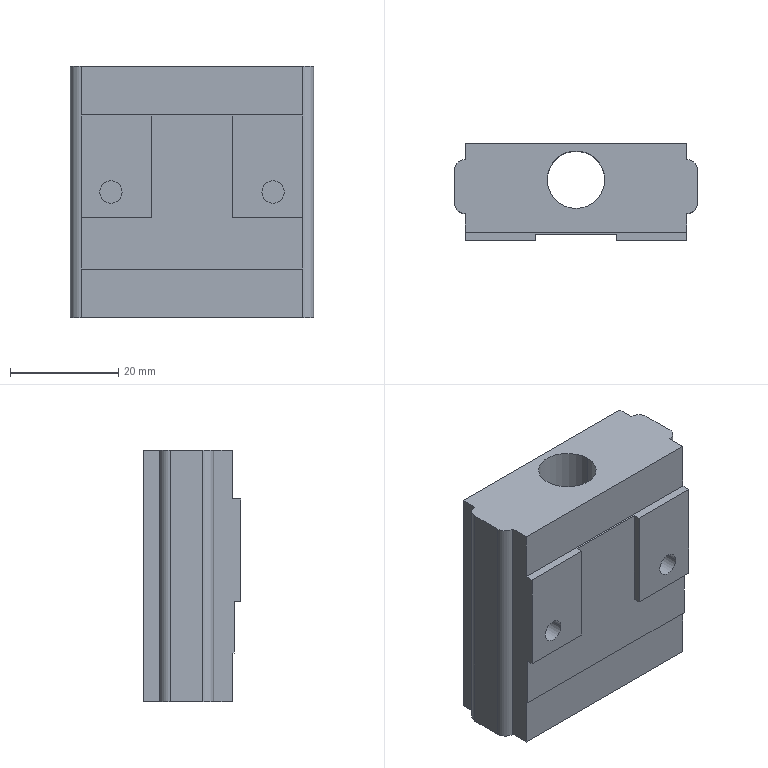Part | SolidWorks | features BaseBody 1 | 1 solid | 32 faces | box 45 x 18 x 46.5 mm | volume 29745 mm3 | plane 22 | cylinder 10 | commonest cylinder face diameters 4 x4 4.134 x4 10.648 x2
STEP:
#1=CARTESIAN_POINT('',(5.831,-18.533,0.));
#2=VERTEX_POINT('',#1);
#3=CARTESIAN_POINT('',(-4.817,-18.533,0.));
#4=VERTEX_POINT('',#3);
#5=CARTESIAN_POINT('',(0.5072,-18.533,0.));
#6=DIRECTION('',(0.,0.,-1.));
#7=DIRECTION('',(1.,0.,0.));
#8=AXIS2_PLACEMENT_3D('',#5,#6,#7);
#9=CIRCLE('',#8,5.324);
#10=EDGE_CURVE('',#2,#4,#9,.T.);
#11=ORIENTED_EDGE('',*,*,#10,.T.);
#12=CARTESIAN_POINT('',(-4.817,-18.533,46.5));
#13=VERTEX_POINT('',#12);
#14=CARTESIAN_POINT('',(-4.817,-18.533,0.));
#15=DIRECTION('',(0.,0.,1.));
#16=VECTOR('',#15,1000.);
#17=LINE('',#14,#16);
#18=EDGE_CURVE('',#4,#13,#17,.T.);
#19=ORIENTED_EDGE('',*,*,#18,.T.);
#20=CARTESIAN_POINT('',(5.831,-18.533,46.5));
#21=VERTEX_POINT('',#20);
#22=CARTESIAN_POINT('',(0.5072,-18.533,46.5));
#23=DIRECTION('',(0.,0.,-1.));
#24=DIRECTION('',(1.,0.,0.));
#25=AXIS2_PLACEMENT_3D('',#22,#23,#24);
#26=CIRCLE('',#25,5.324);
#27=EDGE_CURVE('',#21,#13,#26,.T.);
#28=ORIENTED_EDGE('',*,*,#27,.F.);
#29=CARTESIAN_POINT('',(5.831,-18.533,0.));
#30=DIRECTION('',(0.,0.,1.));
#31=VECTOR('',#30,1000.);
#32=LINE('',#29,#31);
#33=EDGE_CURVE('',#2,#21,#32,.T.);
#34=ORIENTED_EDGE('',*,*,#33,.F.);
#35=EDGE_LOOP('',(#11,#19,#28,#34));
#36=FACE_OUTER_BOUND('',#35,.T.);
#37=CARTESIAN_POINT('',(0.5072,-18.533,0.));
#38=DIRECTION('',(0.,0.,1.));
#39=DIRECTION('',(1.,0.,0.));
#40=AXIS2_PLACEMENT_3D('',#37,#38,#39);
#41=CYLINDRICAL_SURFACE('',#40,5.324);
#42=ADVANCED_FACE('',(#36),#41,.F.);
#43=CARTESIAN_POINT('',(13.44,-21.783,23.25));
#44=VERTEX_POINT('',#43);
#45=CARTESIAN_POINT('',(17.574,-21.783,23.25));
#46=VERTEX_POINT('',#45);
#47=CARTESIAN_POINT('',(15.507,-21.783,23.25));
#48=DIRECTION('',(0.,-1.,0.));
#49=DIRECTION('',(1.,0.,0.));
#50=AXIS2_PLACEMENT_3D('',#47,#48,#49);
#51=CIRCLE('',#50,2.067);
#52=EDGE_CURVE('',#44,#46,#51,.T.);
#53=ORIENTED_EDGE('',*,*,#52,.F.);
#54=CARTESIAN_POINT('',(13.44,-29.783,23.25));
#55=VERTEX_POINT('',#54);
#56=CARTESIAN_POINT('',(13.44,-25.783,23.25));
#57=DIRECTION('',(0.,-1.,0.));
#58=VECTOR('',#57,1000.);
#59=LINE('',#56,#58);
#60=EDGE_CURVE('',#44,#55,#59,.T.);
#61=ORIENTED_EDGE('',*,*,#60,.T.);
#62=CARTESIAN_POINT('',(17.574,-29.783,23.25));
#63=VERTEX_POINT('',#62);
#64=CARTESIAN_POINT('',(15.507,-29.783,23.25));
#65=DIRECTION('',(0.,-1.,0.));
#66=DIRECTION('',(1.,0.,0.));
#67=AXIS2_PLACEMENT_3D('',#64,#65,#66);
#68=CIRCLE('',#67,2.067);
#69=EDGE_CURVE('',#55,#63,#68,.T.);
#70=ORIENTED_EDGE('',*,*,#69,.T.);
#71=CARTESIAN_POINT('',(17.574,-25.783,23.25));
#72=DIRECTION('',(0.,-1.,0.));
#73=VECTOR('',#72,1000.);
#74=LINE('',#71,#73);
#75=EDGE_CURVE('',#46,#63,#74,.T.);
#76=ORIENTED_EDGE('',*,*,#75,.F.);
#77=EDGE_LOOP('',(#53,#61,#70,#76));
#78=FACE_OUTER_BOUND('',#77,.T.);
#79=CARTESIAN_POINT('',(15.507,-25.783,23.25));
#80=DIRECTION('',(0.,-1.,0.));
#81=DIRECTION('',(1.,0.,0.));
#82=AXIS2_PLACEMENT_3D('',#79,#80,#81);
#83=CYLINDRICAL_SURFACE('',#82,2.067);
#84=ADVANCED_FACE('',(#78),#83,.F.);
#85=CARTESIAN_POINT('',(-16.56,-21.783,23.25));
#86=VERTEX_POINT('',#85);
#87=CARTESIAN_POINT('',(-12.426,-21.783,23.25));
#88=VERTEX_POINT('',#87);
#89=CARTESIAN_POINT('',(-14.493,-21.783,23.25));
#90=DIRECTION('',(0.,-1.,0.));
#91=DIRECTION('',(1.,0.,0.));
#92=AXIS2_PLACEMENT_3D('',#89,#90,#91);
#93=CIRCLE('',#92,2.067);
#94=EDGE_CURVE('',#86,#88,#93,.T.);
#95=ORIENTED_EDGE('',*,*,#94,.F.);
#96=CARTESIAN_POINT('',(-16.56,-29.783,23.25));
#97=VERTEX_POINT('',#96);
#98=CARTESIAN_POINT('',(-16.56,-25.783,23.25));
#99=DIRECTION('',(0.,-1.,0.));
#100=VECTOR('',#99,1000.);
#101=LINE('',#98,#100);
#102=EDGE_CURVE('',#86,#97,#101,.T.);
#103=ORIENTED_EDGE('',*,*,#102,.T.);
#104=CARTESIAN_POINT('',(-12.426,-29.783,23.25));
#105=VERTEX_POINT('',#104);
#106=CARTESIAN_POINT('',(-14.493,-29.783,23.25));
#107=DIRECTION('',(0.,-1.,0.));
#108=DIRECTION('',(1.,0.,0.));
#109=AXIS2_PLACEMENT_3D('',#106,#107,#108);
#110=CIRCLE('',#109,2.067);
#111=EDGE_CURVE('',#97,#105,#110,.T.);
#112=ORIENTED_EDGE('',*,*,#111,.T.);
#113=CARTESIAN_POINT('',(-12.426,-25.783,23.25));
#114=DIRECTION('',(0.,-1.,0.));
#115=VECTOR('',#114,1000.);
#116=LINE('',#113,#115);
#117=EDGE_CURVE('',#88,#105,#116,.T.);
#118=ORIENTED_EDGE('',*,*,#117,.F.);
#119=EDGE_LOOP('',(#95,#103,#112,#118));
#120=FACE_OUTER_BOUND('',#119,.T.);
#121=CARTESIAN_POINT('',(-14.493,-25.783,23.25));
#122=DIRECTION('',(0.,-1.,0.));
#123=DIRECTION('',(1.,0.,0.));
#124=AXIS2_PLACEMENT_3D('',#121,#122,#123);
#125=CYLINDRICAL_SURFACE('',#124,2.067);
#126=ADVANCED_FACE('',(#120),#125,.F.);
#127=CARTESIAN_POINT('',(21.007,-11.783,0.));
#128=VERTEX_POINT('',#127);
#129=CARTESIAN_POINT('',(-19.993,-11.783,0.));
#130=VERTEX_POINT('',#129);
#131=CARTESIAN_POINT('',(-19.993,-11.783,0.));
#132=DIRECTION('',(-1.,0.,0.));
#133=VECTOR('',#132,1000.);
#134=LINE('',#131,#133);
#135=EDGE_CURVE('',#128,#130,#134,.T.);
#136=ORIENTED_EDGE('',*,*,#135,.T.);
#137=CARTESIAN_POINT('',(-19.993,-11.783,46.5));
#138=VERTEX_POINT('',#137);
#139=CARTESIAN_POINT('',(-19.993,-11.783,0.));
#140=DIRECTION('',(0.,0.,1.));
#141=VECTOR('',#140,1000.);
#142=LINE('',#139,#141);
#143=EDGE_CURVE('',#130,#138,#142,.T.);
#144=ORIENTED_EDGE('',*,*,#143,.T.);
#145=CARTESIAN_POINT('',(21.007,-11.783,46.5));
#146=VERTEX_POINT('',#145);
#147=CARTESIAN_POINT('',(-19.993,-11.783,46.5));
#148=DIRECTION('',(1.,0.,0.));
#149=VECTOR('',#148,1000.);
#150=LINE('',#147,#149);
#151=EDGE_CURVE('',#138,#146,#150,.T.);
#152=ORIENTED_EDGE('',*,*,#151,.T.);
#153=CARTESIAN_POINT('',(21.007,-11.783,0.));
#154=DIRECTION('',(0.,0.,-1.));
#155=VECTOR('',#154,1000.);
#156=LINE('',#153,#155);
#157=EDGE_CURVE('',#146,#128,#156,.T.);
#158=ORIENTED_EDGE('',*,*,#157,.T.);
#159=EDGE_LOOP('',(#136,#144,#152,#158));
#160=FACE_OUTER_BOUND('',#159,.T.);
#161=CARTESIAN_POINT('',(-19.993,-11.783,0.));
#162=DIRECTION('',(0.,1.,0.));
#163=DIRECTION('',(0.,0.,1.));
#164=AXIS2_PLACEMENT_3D('',#161,#162,#163);
#165=PLANE('',#164);
#166=ADVANCED_FACE('',(#160),#165,.T.);
#167=ORIENTED_EDGE('',*,*,#143,.F.);
#168=CARTESIAN_POINT('',(-19.993,-14.783,0.));
#169=VERTEX_POINT('',#168);
#170=CARTESIAN_POINT('',(-19.993,-16.783,0.));
#171=DIRECTION('',(0.,-1.,0.));
#172=VECTOR('',#171,1000.);
#173=LINE('',#170,#172);
#174=EDGE_CURVE('',#130,#169,#173,.T.);
#175=ORIENTED_EDGE('',*,*,#174,.T.);
#176=CARTESIAN_POINT('',(-19.993,-14.783,46.5));
#177=VERTEX_POINT('',#176);
#178=CARTESIAN_POINT('',(-19.993,-14.783,0.));
#179=DIRECTION('',(0.,0.,1.));
#180=VECTOR('',#179,1000.);
#181=LINE('',#178,#180);
#182=EDGE_CURVE('',#169,#177,#181,.T.);
#183=ORIENTED_EDGE('',*,*,#182,.T.);
#184=CARTESIAN_POINT('',(-19.993,-16.783,46.5));
#185=DIRECTION('',(0.,1.,0.));
#186=VECTOR('',#185,1000.);
#187=LINE('',#184,#186);
#188=EDGE_CURVE('',#177,#138,#187,.T.);
#189=ORIENTED_EDGE('',*,*,#188,.T.);
#190=EDGE_LOOP('',(#167,#175,#183,#189));
#191=FACE_OUTER_BOUND('',#190,.T.);
#192=CARTESIAN_POINT('',(-19.993,-16.783,0.));
#193=DIRECTION('',(-1.,0.,0.));
#194=DIRECTION('',(0.,0.,1.));
#195=AXIS2_PLACEMENT_3D('',#192,#193,#194);
#196=PLANE('',#195);
#197=ADVANCED_FACE('',(#191),#196,.T.);
#198=ORIENTED_EDGE('',*,*,#10,.F.);
#199=CARTESIAN_POINT('',(0.5072,-18.533,0.));
#200=DIRECTION('',(0.,0.,-1.));
#201=DIRECTION('',(1.,0.,0.));
#202=AXIS2_PLACEMENT_3D('',#199,#200,#201);
#203=CIRCLE('',#202,5.324);
#204=EDGE_CURVE('',#4,#2,#203,.T.);
#205=ORIENTED_EDGE('',*,*,#204,.F.);
#206=EDGE_LOOP('',(#198,#205));
#207=FACE_BOUND('',#206,.T.);
#208=CARTESIAN_POINT('',(23.007,-22.783,0.));
#209=VERTEX_POINT('',#208);
#210=CARTESIAN_POINT('',(23.007,-16.783,0.));
#211=VERTEX_POINT('',#210);
#212=CARTESIAN_POINT('',(23.007,-19.783,0.));
#213=DIRECTION('',(0.,1.,0.));
#214=VECTOR('',#213,1000.);
#215=LINE('',#212,#214);
#216=EDGE_CURVE('',#209,#211,#215,.T.);
#217=ORIENTED_EDGE('',*,*,#216,.F.);
#218=CARTESIAN_POINT('',(21.007,-24.783,0.));
#219=VERTEX_POINT('',#218);
#220=CARTESIAN_POINT('',(21.007,-22.783,0.));
#221=DIRECTION('',(0.,0.,1.));
#222=DIRECTION('',(1.,0.,0.));
#223=AXIS2_PLACEMENT_3D('',#220,#221,#222);
#224=CIRCLE('',#223,2.);
#225=EDGE_CURVE('',#219,#209,#224,.T.);
#226=ORIENTED_EDGE('',*,*,#225,.F.);
#227=CARTESIAN_POINT('',(21.007,-28.283,0.));
#228=VERTEX_POINT('',#227);
#229=CARTESIAN_POINT('',(21.007,-19.783,0.));
#230=DIRECTION('',(0.,1.,0.));
#231=VECTOR('',#230,1000.);
#232=LINE('',#229,#231);
#233=EDGE_CURVE('',#228,#219,#232,.T.);
#234=ORIENTED_EDGE('',*,*,#233,.F.);
#235=CARTESIAN_POINT('',(-19.993,-28.283,0.));
#236=VERTEX_POINT('',#235);
#237=CARTESIAN_POINT('',(0.5072,-28.283,0.));
#238=DIRECTION('',(1.,0.,0.));
#239=VECTOR('',#238,1000.);
#240=LINE('',#237,#239);
#241=EDGE_CURVE('',#236,#228,#240,.T.);
#242=ORIENTED_EDGE('',*,*,#241,.F.);
#243=CARTESIAN_POINT('',(-19.993,-24.783,0.));
#244=VERTEX_POINT('',#243);
#245=CARTESIAN_POINT('',(-19.993,-19.783,0.));
#246=DIRECTION('',(0.,-1.,0.));
#247=VECTOR('',#246,1000.);
#248=LINE('',#245,#247);
#249=EDGE_CURVE('',#244,#236,#248,.T.);
#250=ORIENTED_EDGE('',*,*,#249,.F.);
#251=CARTESIAN_POINT('',(-21.993,-22.783,0.));
#252=VERTEX_POINT('',#251);
#253=CARTESIAN_POINT('',(-19.993,-22.783,0.));
#254=DIRECTION('',(0.,0.,1.));
#255=DIRECTION('',(1.,0.,0.));
#256=AXIS2_PLACEMENT_3D('',#253,#254,#255);
#257=CIRCLE('',#256,2.);
#258=EDGE_CURVE('',#252,#244,#257,.T.);
#259=ORIENTED_EDGE('',*,*,#258,.F.);
#260=CARTESIAN_POINT('',(-21.993,-16.783,0.));
#261=VERTEX_POINT('',#260);
#262=CARTESIAN_POINT('',(-21.993,-19.783,0.));
#263=DIRECTION('',(0.,-1.,0.));
#264=VECTOR('',#263,1000.);
#265=LINE('',#262,#264);
#266=EDGE_CURVE('',#261,#252,#265,.T.);
#267=ORIENTED_EDGE('',*,*,#266,.F.);
#268=CARTESIAN_POINT('',(-19.993,-16.783,0.));
#269=DIRECTION('',(0.,0.,1.));
#270=DIRECTION('',(1.,0.,0.));
#271=AXIS2_PLACEMENT_3D('',#268,#269,#270);
#272=CIRCLE('',#271,2.);
#273=EDGE_CURVE('',#169,#261,#272,.T.);
#274=ORIENTED_EDGE('',*,*,#273,.F.);
#275=ORIENTED_EDGE('',*,*,#174,.F.);
#276=ORIENTED_EDGE('',*,*,#135,.F.);
#277=CARTESIAN_POINT('',(21.007,-14.783,0.));
#278=VERTEX_POINT('',#277);
#279=CARTESIAN_POINT('',(21.007,-19.783,0.));
#280=DIRECTION('',(0.,1.,0.));
#281=VECTOR('',#280,1000.);
#282=LINE('',#279,#281);
#283=EDGE_CURVE('',#278,#128,#282,.T.);
#284=ORIENTED_EDGE('',*,*,#283,.F.);
#285=CARTESIAN_POINT('',(21.007,-16.783,0.));
#286=DIRECTION('',(0.,0.,1.));
#287=DIRECTION('',(1.,0.,0.));
#288=AXIS2_PLACEMENT_3D('',#285,#286,#287);
#289=CIRCLE('',#288,2.);
#290=EDGE_CURVE('',#211,#278,#289,.T.);
#291=ORIENTED_EDGE('',*,*,#290,.F.);
#292=EDGE_LOOP('',(#217,#226,#234,#242,#250,#259,#267,#274,#275,#276,#284,#291));
#293=FACE_OUTER_BOUND('',#292,.T.);
#294=CARTESIAN_POINT('',(0.5072,-19.783,0.));
#295=DIRECTION('',(0.,0.,1.));
#296=DIRECTION('',(1.,0.,0.));
#297=AXIS2_PLACEMENT_3D('',#294,#295,#296);
#298=PLANE('',#297);
#299=ADVANCED_FACE('',(#207,#293),#298,.F.);
#300=ORIENTED_EDGE('',*,*,#157,.F.);
#301=CARTESIAN_POINT('',(21.007,-14.783,46.5));
#302=VERTEX_POINT('',#301);
#303=CARTESIAN_POINT('',(21.007,-11.783,46.5));
#304=DIRECTION('',(0.,-1.,0.));
#305=VECTOR('',#304,1000.);
#306=LINE('',#303,#305);
#307=EDGE_CURVE('',#146,#302,#306,.T.);
#308=ORIENTED_EDGE('',*,*,#307,.T.);
#309=CARTESIAN_POINT('',(21.007,-14.783,0.));
#310=DIRECTION('',(0.,0.,-1.));
#311=VECTOR('',#310,1000.);
#312=LINE('',#309,#311);
#313=EDGE_CURVE('',#302,#278,#312,.T.);
#314=ORIENTED_EDGE('',*,*,#313,.T.);
#315=ORIENTED_EDGE('',*,*,#283,.T.);
#316=EDGE_LOOP('',(#300,#308,#314,#315));
#317=FACE_OUTER_BOUND('',#316,.T.);
#318=CARTESIAN_POINT('',(21.007,-11.783,0.));
#319=DIRECTION('',(1.,0.,0.));
#320=DIRECTION('',(0.,0.,-1.));
#321=AXIS2_PLACEMENT_3D('',#318,#319,#320);
#322=PLANE('',#321);
#323=ADVANCED_FACE('',(#317),#322,.T.);
#324=ORIENTED_EDGE('',*,*,#27,.T.);
#325=CARTESIAN_POINT('',(0.5072,-18.533,46.5));
#326=DIRECTION('',(0.,0.,-1.));
#327=DIRECTION('',(1.,0.,0.));
#328=AXIS2_PLACEMENT_3D('',#325,#326,#327);
#329=CIRCLE('',#328,5.324);
#330=EDGE_CURVE('',#13,#21,#329,.T.);
#331=ORIENTED_EDGE('',*,*,#330,.T.);
#332=EDGE_LOOP('',(#324,#331));
#333=FACE_BOUND('',#332,.T.);
#334=ORIENTED_EDGE('',*,*,#151,.F.);
#335=ORIENTED_EDGE('',*,*,#188,.F.);
#336=CARTESIAN_POINT('',(-21.993,-16.783,46.5));
#337=VERTEX_POINT('',#336);
#338=CARTESIAN_POINT('',(-19.993,-16.783,46.5));
#339=DIRECTION('',(0.,0.,1.));
#340=DIRECTION('',(1.,0.,0.));
#341=AXIS2_PLACEMENT_3D('',#338,#339,#340);
#342=CIRCLE('',#341,2.);
#343=EDGE_CURVE('',#177,#337,#342,.T.);
#344=ORIENTED_EDGE('',*,*,#343,.T.);
#345=CARTESIAN_POINT('',(-21.993,-22.783,46.5));
#346=VERTEX_POINT('',#345);
#347=CARTESIAN_POINT('',(-21.993,-19.783,46.5));
#348=DIRECTION('',(0.,-1.,0.));
#349=VECTOR('',#348,1000.);
#350=LINE('',#347,#349);
#351=EDGE_CURVE('',#337,#346,#350,.T.);
#352=ORIENTED_EDGE('',*,*,#351,.T.);
#353=CARTESIAN_POINT('',(-19.993,-24.783,46.5));
#354=VERTEX_POINT('',#353);
#355=CARTESIAN_POINT('',(-19.993,-22.783,46.5));
#356=DIRECTION('',(0.,0.,1.));
#357=DIRECTION('',(1.,0.,0.));
#358=AXIS2_PLACEMENT_3D('',#355,#356,#357);
#359=CIRCLE('',#358,2.);
#360=EDGE_CURVE('',#346,#354,#359,.T.);
#361=ORIENTED_EDGE('',*,*,#360,.T.);
#362=CARTESIAN_POINT('',(-19.993,-28.283,46.5));
#363=VERTEX_POINT('',#362);
#364=CARTESIAN_POINT('',(-19.993,-19.783,46.5));
#365=DIRECTION('',(0.,-1.,0.));
#366=VECTOR('',#365,1000.);
#367=LINE('',#364,#366);
#368=EDGE_CURVE('',#354,#363,#367,.T.);
#369=ORIENTED_EDGE('',*,*,#368,.T.);
#370=CARTESIAN_POINT('',(21.007,-28.283,46.5));
#371=VERTEX_POINT('',#370);
#372=CARTESIAN_POINT('',(0.5072,-28.283,46.5));
#373=DIRECTION('',(1.,0.,0.));
#374=VECTOR('',#373,1000.);
#375=LINE('',#372,#374);
#376=EDGE_CURVE('',#363,#371,#375,.T.);
#377=ORIENTED_EDGE('',*,*,#376,.T.);
#378=CARTESIAN_POINT('',(21.007,-24.783,46.5));
#379=VERTEX_POINT('',#378);
#380=CARTESIAN_POINT('',(21.007,-19.783,46.5));
#381=DIRECTION('',(0.,1.,0.));
#382=VECTOR('',#381,1000.);
#383=LINE('',#380,#382);
#384=EDGE_CURVE('',#371,#379,#383,.T.);
#385=ORIENTED_EDGE('',*,*,#384,.T.);
#386=CARTESIAN_POINT('',(23.007,-22.783,46.5));
#387=VERTEX_POINT('',#386);
#388=CARTESIAN_POINT('',(21.007,-22.783,46.5));
#389=DIRECTION('',(0.,0.,1.));
#390=DIRECTION('',(1.,0.,0.));
#391=AXIS2_PLACEMENT_3D('',#388,#389,#390);
#392=CIRCLE('',#391,2.);
#393=EDGE_CURVE('',#379,#387,#392,.T.);
#394=ORIENTED_EDGE('',*,*,#393,.T.);
#395=CARTESIAN_POINT('',(23.007,-16.783,46.5));
#396=VERTEX_POINT('',#395);
#397=CARTESIAN_POINT('',(23.007,-19.783,46.5));
#398=DIRECTION('',(0.,1.,0.));
#399=VECTOR('',#398,1000.);
#400=LINE('',#397,#399);
#401=EDGE_CURVE('',#387,#396,#400,.T.);
#402=ORIENTED_EDGE('',*,*,#401,.T.);
#403=CARTESIAN_POINT('',(21.007,-16.783,46.5));
#404=DIRECTION('',(0.,0.,1.));
#405=DIRECTION('',(1.,0.,0.));
#406=AXIS2_PLACEMENT_3D('',#403,#404,#405);
#407=CIRCLE('',#406,2.);
#408=EDGE_CURVE('',#396,#302,#407,.T.);
#409=ORIENTED_EDGE('',*,*,#408,.T.);
#410=ORIENTED_EDGE('',*,*,#307,.F.);
#411=EDGE_LOOP('',(#334,#335,#344,#352,#361,#369,#377,#385,#394,#402,#409,#410));
#412=FACE_OUTER_BOUND('',#411,.T.);
#413=CARTESIAN_POINT('',(0.5072,-19.783,46.5));
#414=DIRECTION('',(0.,0.,1.));
#415=DIRECTION('',(1.,0.,0.));
#416=AXIS2_PLACEMENT_3D('',#413,#414,#415);
#417=PLANE('',#416);
#418=ADVANCED_FACE('',(#333,#412),#417,.T.);
#419=ORIENTED_EDGE('',*,*,#273,.T.);
#420=CARTESIAN_POINT('',(-21.993,-16.783,0.));
#421=DIRECTION('',(0.,0.,1.));
#422=VECTOR('',#421,1000.);
#423=LINE('',#420,#422);
#424=EDGE_CURVE('',#261,#337,#423,.T.);
#425=ORIENTED_EDGE('',*,*,#424,.T.);
#426=ORIENTED_EDGE('',*,*,#343,.F.);
#427=ORIENTED_EDGE('',*,*,#182,.F.);
#428=EDGE_LOOP('',(#419,#425,#426,#427));
#429=FACE_OUTER_BOUND('',#428,.T.);
#430=CARTESIAN_POINT('',(-19.993,-16.783,0.));
#431=DIRECTION('',(0.,0.,1.));
#432=DIRECTION('',(1.,0.,0.));
#433=AXIS2_PLACEMENT_3D('',#430,#431,#432);
#434=CYLINDRICAL_SURFACE('',#433,2.);
#435=ADVANCED_FACE('',(#429),#434,.T.);
#436=ORIENTED_EDGE('',*,*,#18,.F.);
#437=ORIENTED_EDGE('',*,*,#204,.T.);
#438=ORIENTED_EDGE('',*,*,#33,.T.);
#439=ORIENTED_EDGE('',*,*,#330,.F.);
#440=EDGE_LOOP('',(#436,#437,#438,#439));
#441=FACE_OUTER_BOUND('',#440,.T.);
#442=CARTESIAN_POINT('',(0.5072,-18.533,0.));
#443=DIRECTION('',(0.,0.,1.));
#444=DIRECTION('',(1.,0.,0.));
#445=AXIS2_PLACEMENT_3D('',#442,#443,#444);
#446=CYLINDRICAL_SURFACE('',#445,5.324);
#447=ADVANCED_FACE('',(#441),#446,.F.);
#448=ORIENTED_EDGE('',*,*,#290,.T.);
#449=ORIENTED_EDGE('',*,*,#313,.F.);
#450=ORIENTED_EDGE('',*,*,#408,.F.);
#451=CARTESIAN_POINT('',(23.007,-16.783,0.));
#452=DIRECTION('',(0.,0.,-1.));
#453=VECTOR('',#452,1000.);
#454=LINE('',#451,#453);
#455=EDGE_CURVE('',#396,#211,#454,.T.);
#456=ORIENTED_EDGE('',*,*,#455,.T.);
#457=EDGE_LOOP('',(#448,#449,#450,#456));
#458=FACE_OUTER_BOUND('',#457,.T.);
#459=CARTESIAN_POINT('',(21.007,-16.783,0.));
#460=DIRECTION('',(0.,0.,1.));
#461=DIRECTION('',(1.,0.,0.));
#462=AXIS2_PLACEMENT_3D('',#459,#460,#461);
#463=CYLINDRICAL_SURFACE('',#462,2.);
#464=ADVANCED_FACE('',(#458),#463,.T.);
#465=CARTESIAN_POINT('',(23.007,-22.783,0.));
#466=DIRECTION('',(0.,0.,-1.));
#467=VECTOR('',#466,1000.);
#468=LINE('',#465,#467);
#469=EDGE_CURVE('',#387,#209,#468,.T.);
#470=ORIENTED_EDGE('',*,*,#469,.T.);
#471=ORIENTED_EDGE('',*,*,#216,.T.);
#472=ORIENTED_EDGE('',*,*,#455,.F.);
#473=ORIENTED_EDGE('',*,*,#401,.F.);
#474=EDGE_LOOP('',(#470,#471,#472,#473));
#475=FACE_OUTER_BOUND('',#474,.T.);
#476=CARTESIAN_POINT('',(23.007,-14.783,0.));
#477=DIRECTION('',(1.,0.,0.));
#478=DIRECTION('',(0.,0.,-1.));
#479=AXIS2_PLACEMENT_3D('',#476,#477,#478);
#480=PLANE('',#479);
#481=ADVANCED_FACE('',(#475),#480,.T.);
#482=ORIENTED_EDGE('',*,*,#225,.T.);
#483=ORIENTED_EDGE('',*,*,#469,.F.);
#484=ORIENTED_EDGE('',*,*,#393,.F.);
#485=CARTESIAN_POINT('',(21.007,-24.783,0.));
#486=DIRECTION('',(0.,0.,-1.));
#487=VECTOR('',#486,1000.);
#488=LINE('',#485,#487);
#489=EDGE_CURVE('',#379,#219,#488,.T.);
#490=ORIENTED_EDGE('',*,*,#489,.T.);
#491=EDGE_LOOP('',(#482,#483,#484,#490));
#492=FACE_OUTER_BOUND('',#491,.T.);
#493=CARTESIAN_POINT('',(21.007,-22.783,0.));
#494=DIRECTION('',(0.,0.,1.));
#495=DIRECTION('',(1.,0.,0.));
#496=AXIS2_PLACEMENT_3D('',#493,#494,#495);
#497=CYLINDRICAL_SURFACE('',#496,2.);
#498=ADVANCED_FACE('',(#492),#497,.T.);
#499=CARTESIAN_POINT('',(21.007,-29.783,37.5));
#500=VERTEX_POINT('',#499);
#501=CARTESIAN_POINT('',(21.007,-29.783,18.5));
#502=VERTEX_POINT('',#501);
#503=CARTESIAN_POINT('',(21.007,-29.783,46.5));
#504=DIRECTION('',(0.,0.,-1.));
#505=VECTOR('',#504,1000.);
#506=LINE('',#503,#505);
#507=EDGE_CURVE('',#500,#502,#506,.T.);
#508=ORIENTED_EDGE('',*,*,#507,.T.);
#509=CARTESIAN_POINT('',(21.007,-28.583,18.5));
#510=VERTEX_POINT('',#509);
#511=CARTESIAN_POINT('',(21.007,-29.783,18.5));
#512=DIRECTION('',(0.,1.,0.));
#513=VECTOR('',#512,1000.);
#514=LINE('',#511,#513);
#515=EDGE_CURVE('',#502,#510,#514,.T.);
#516=ORIENTED_EDGE('',*,*,#515,.T.);
#517=CARTESIAN_POINT('',(21.007,-28.583,9.));
#518=VERTEX_POINT('',#517);
#519=CARTESIAN_POINT('',(21.007,-28.583,46.5));
#520=DIRECTION('',(0.,0.,-1.));
#521=VECTOR('',#520,1000.);
#522=LINE('',#519,#521);
#523=EDGE_CURVE('',#510,#518,#522,.T.);
#524=ORIENTED_EDGE('',*,*,#523,.T.);
#525=CARTESIAN_POINT('',(21.007,-28.283,9.));
#526=VERTEX_POINT('',#525);
#527=CARTESIAN_POINT('',(21.007,-29.783,9.));
#528=DIRECTION('',(0.,-1.,0.));
#529=VECTOR('',#528,1000.);
#530=LINE('',#527,#529);
#531=EDGE_CURVE('',#526,#518,#530,.T.);
#532=ORIENTED_EDGE('',*,*,#531,.F.);
#533=CARTESIAN_POINT('',(21.007,-28.283,46.5));
#534=DIRECTION('',(0.,0.,-1.));
#535=VECTOR('',#534,1000.);
#536=LINE('',#533,#535);
#537=EDGE_CURVE('',#526,#228,#536,.T.);
#538=ORIENTED_EDGE('',*,*,#537,.T.);
#539=ORIENTED_EDGE('',*,*,#233,.T.);
#540=ORIENTED_EDGE('',*,*,#489,.F.);
#541=ORIENTED_EDGE('',*,*,#384,.F.);
#542=CARTESIAN_POINT('',(21.007,-28.283,37.5));
#543=VERTEX_POINT('',#542);
#544=CARTESIAN_POINT('',(21.007,-28.283,46.5));
#545=DIRECTION('',(0.,0.,-1.));
#546=VECTOR('',#545,1000.);
#547=LINE('',#544,#546);
#548=EDGE_CURVE('',#371,#543,#547,.T.);
#549=ORIENTED_EDGE('',*,*,#548,.T.);
#550=CARTESIAN_POINT('',(21.007,-29.783,37.5));
#551=DIRECTION('',(0.,1.,0.));
#552=VECTOR('',#551,1000.);
#553=LINE('',#550,#552);
#554=EDGE_CURVE('',#500,#543,#553,.T.);
#555=ORIENTED_EDGE('',*,*,#554,.F.);
#556=EDGE_LOOP('',(#508,#516,#524,#532,#538,#539,#540,#541,#549,#555));
#557=FACE_OUTER_BOUND('',#556,.T.);
#558=CARTESIAN_POINT('',(21.007,-24.783,46.5));
#559=DIRECTION('',(1.,0.,0.));
#560=DIRECTION('',(0.,0.,-1.));
#561=AXIS2_PLACEMENT_3D('',#558,#559,#560);
#562=PLANE('',#561);
#563=ADVANCED_FACE('',(#557),#562,.T.);
#564=CARTESIAN_POINT('',(-19.993,-28.283,9.));
#565=VERTEX_POINT('',#564);
#566=CARTESIAN_POINT('',(-19.993,-28.283,23.25));
#567=DIRECTION('',(0.,0.,1.));
#568=VECTOR('',#567,1000.);
#569=LINE('',#566,#568);
#570=EDGE_CURVE('',#236,#565,#569,.T.);
#571=ORIENTED_EDGE('',*,*,#570,.F.);
#572=ORIENTED_EDGE('',*,*,#241,.T.);
#573=ORIENTED_EDGE('',*,*,#537,.F.);
#574=CARTESIAN_POINT('',(0.5072,-28.283,9.));
#575=DIRECTION('',(1.,0.,0.));
#576=VECTOR('',#575,1000.);
#577=LINE('',#574,#576);
#578=EDGE_CURVE('',#565,#526,#577,.T.);
#579=ORIENTED_EDGE('',*,*,#578,.F.);
#580=EDGE_LOOP('',(#571,#572,#573,#579));
#581=FACE_OUTER_BOUND('',#580,.T.);
#582=CARTESIAN_POINT('',(0.5072,-28.283,23.25));
#583=DIRECTION('',(0.,1.,0.));
#584=DIRECTION('',(0.,0.,1.));
#585=AXIS2_PLACEMENT_3D('',#582,#583,#584);
#586=PLANE('',#585);
#587=ADVANCED_FACE('',(#581),#586,.F.);
#588=ORIENTED_EDGE('',*,*,#570,.T.);
#589=CARTESIAN_POINT('',(-19.993,-28.583,9.));
#590=VERTEX_POINT('',#589);
#591=CARTESIAN_POINT('',(-19.993,-24.783,9.));
#592=DIRECTION('',(0.,-1.,0.));
#593=VECTOR('',#592,1000.);
#594=LINE('',#591,#593);
#595=EDGE_CURVE('',#565,#590,#594,.T.);
#596=ORIENTED_EDGE('',*,*,#595,.T.);
#597=CARTESIAN_POINT('',(-19.993,-28.583,18.5));
#598=VERTEX_POINT('',#597);
#599=CARTESIAN_POINT('',(-19.993,-28.583,0.));
#600=DIRECTION('',(0.,0.,1.));
#601=VECTOR('',#600,1000.);
#602=LINE('',#599,#601);
#603=EDGE_CURVE('',#590,#598,#602,.T.);
#604=ORIENTED_EDGE('',*,*,#603,.T.);
#605=CARTESIAN_POINT('',(-19.993,-29.783,18.5));
#606=VERTEX_POINT('',#605);
#607=CARTESIAN_POINT('',(-19.993,-29.783,18.5));
#608=DIRECTION('',(0.,-1.,0.));
#609=VECTOR('',#608,1000.);
#610=LINE('',#607,#609);
#611=EDGE_CURVE('',#598,#606,#610,.T.);
#612=ORIENTED_EDGE('',*,*,#611,.T.);
#613=CARTESIAN_POINT('',(-19.993,-29.783,37.5));
#614=VERTEX_POINT('',#613);
#615=CARTESIAN_POINT('',(-19.993,-29.783,0.));
#616=DIRECTION('',(0.,0.,1.));
#617=VECTOR('',#616,1000.);
#618=LINE('',#615,#617);
#619=EDGE_CURVE('',#606,#614,#618,.T.);
#620=ORIENTED_EDGE('',*,*,#619,.T.);
#621=CARTESIAN_POINT('',(-19.993,-28.283,37.5));
#622=VERTEX_POINT('',#621);
#623=CARTESIAN_POINT('',(-19.993,-29.783,37.5));
#624=DIRECTION('',(0.,-1.,0.));
#625=VECTOR('',#624,1000.);
#626=LINE('',#623,#625);
#627=EDGE_CURVE('',#622,#614,#626,.T.);
#628=ORIENTED_EDGE('',*,*,#627,.F.);
#629=CARTESIAN_POINT('',(-19.993,-28.283,0.));
#630=DIRECTION('',(0.,0.,1.));
#631=VECTOR('',#630,1000.);
#632=LINE('',#629,#631);
#633=EDGE_CURVE('',#622,#363,#632,.T.);
#634=ORIENTED_EDGE('',*,*,#633,.T.);
#635=ORIENTED_EDGE('',*,*,#368,.F.);
#636=CARTESIAN_POINT('',(-19.993,-24.783,0.));
#637=DIRECTION('',(0.,0.,-1.));
#638=VECTOR('',#637,1000.);
#639=LINE('',#636,#638);
#640=EDGE_CURVE('',#354,#244,#639,.T.);
#641=ORIENTED_EDGE('',*,*,#640,.T.);
#642=ORIENTED_EDGE('',*,*,#249,.T.);
#643=EDGE_LOOP('',(#588,#596,#604,#612,#620,#628,#634,#635,#641,#642));
#644=FACE_OUTER_BOUND('',#643,.T.);
#645=CARTESIAN_POINT('',(-19.993,-24.783,0.));
#646=DIRECTION('',(-1.,0.,0.));
#647=DIRECTION('',(0.,0.,1.));
#648=AXIS2_PLACEMENT_3D('',#645,#646,#647);
#649=PLANE('',#648);
#650=ADVANCED_FACE('',(#644),#649,.T.);
#651=ORIENTED_EDGE('',*,*,#258,.T.);
#652=ORIENTED_EDGE('',*,*,#640,.F.);
#653=ORIENTED_EDGE('',*,*,#360,.F.);
#654=CARTESIAN_POINT('',(-21.993,-22.783,0.));
#655=DIRECTION('',(0.,0.,-1.));
#656=VECTOR('',#655,1000.);
#657=LINE('',#654,#656);
#658=EDGE_CURVE('',#346,#252,#657,.T.);
#659=ORIENTED_EDGE('',*,*,#658,.T.);
#660=EDGE_LOOP('',(#651,#652,#653,#659));
#661=FACE_OUTER_BOUND('',#660,.T.);
#662=CARTESIAN_POINT('',(-19.993,-22.783,0.));
#663=DIRECTION('',(0.,0.,1.));
#664=DIRECTION('',(1.,0.,0.));
#665=AXIS2_PLACEMENT_3D('',#662,#663,#664);
#666=CYLINDRICAL_SURFACE('',#665,2.);
#667=ADVANCED_FACE('',(#661),#666,.T.);
#668=ORIENTED_EDGE('',*,*,#424,.F.);
#669=ORIENTED_EDGE('',*,*,#266,.T.);
#670=ORIENTED_EDGE('',*,*,#658,.F.);
#671=ORIENTED_EDGE('',*,*,#351,.F.);
#672=EDGE_LOOP('',(#668,#669,#670,#671));
#673=FACE_OUTER_BOUND('',#672,.T.);
#674=CARTESIAN_POINT('',(-21.993,-24.783,0.));
#675=DIRECTION('',(-1.,0.,0.));
#676=DIRECTION('',(0.,0.,1.));
#677=AXIS2_PLACEMENT_3D('',#674,#675,#676);
#678=PLANE('',#677);
#679=ADVANCED_FACE('',(#673),#678,.T.);
#680=ORIENTED_EDGE('',*,*,#548,.F.);
#681=ORIENTED_EDGE('',*,*,#376,.F.);
#682=ORIENTED_EDGE('',*,*,#633,.F.);
#683=CARTESIAN_POINT('',(0.5072,-28.283,37.5));
#684=DIRECTION('',(-1.,0.,0.));
#685=VECTOR('',#684,1000.);
#686=LINE('',#683,#685);
#687=EDGE_CURVE('',#543,#622,#686,.T.);
#688=ORIENTED_EDGE('',*,*,#687,.F.);
#689=EDGE_LOOP('',(#680,#681,#682,#688));
#690=FACE_OUTER_BOUND('',#689,.T.);
#691=CARTESIAN_POINT('',(0.5072,-28.283,23.25));
#692=DIRECTION('',(0.,1.,0.));
#693=DIRECTION('',(0.,0.,1.));
#694=AXIS2_PLACEMENT_3D('',#691,#692,#693);
#695=PLANE('',#694);
#696=ADVANCED_FACE('',(#690),#695,.F.);
#697=CARTESIAN_POINT('',(15.507,-29.783,23.25));
#698=DIRECTION('',(0.,-1.,0.));
#699=DIRECTION('',(1.,0.,0.));
#700=AXIS2_PLACEMENT_3D('',#697,#698,#699);
#701=CIRCLE('',#700,2.067);
#702=EDGE_CURVE('',#63,#55,#701,.T.);
#703=ORIENTED_EDGE('',*,*,#702,.F.);
#704=ORIENTED_EDGE('',*,*,#69,.F.);
#705=EDGE_LOOP('',(#703,#704));
#706=FACE_BOUND('',#705,.T.);
#707=ORIENTED_EDGE('',*,*,#507,.F.);
#708=CARTESIAN_POINT('',(8.007,-29.783,37.5));
#709=VERTEX_POINT('',#708);
#710=CARTESIAN_POINT('',(0.5072,-29.783,37.5));
#711=DIRECTION('',(1.,0.,0.));
#712=VECTOR('',#711,1000.);
#713=LINE('',#710,#712);
#714=EDGE_CURVE('',#709,#500,#713,.T.);
#715=ORIENTED_EDGE('',*,*,#714,.F.);
#716=CARTESIAN_POINT('',(8.007,-29.783,18.5));
#717=VERTEX_POINT('',#716);
#718=CARTESIAN_POINT('',(8.007,-29.783,23.25));
#719=DIRECTION('',(0.,0.,1.));
#720=VECTOR('',#719,1000.);
#721=LINE('',#718,#720);
#722=EDGE_CURVE('',#717,#709,#721,.T.);
#723=ORIENTED_EDGE('',*,*,#722,.F.);
#724=CARTESIAN_POINT('',(0.5072,-29.783,18.5));
#725=DIRECTION('',(-1.,0.,0.));
#726=VECTOR('',#725,1000.);
#727=LINE('',#724,#726);
#728=EDGE_CURVE('',#502,#717,#727,.T.);
#729=ORIENTED_EDGE('',*,*,#728,.F.);
#730=EDGE_LOOP('',(#707,#715,#723,#729));
#731=FACE_OUTER_BOUND('',#730,.T.);
#732=CARTESIAN_POINT('',(0.5072,-29.783,23.25));
#733=DIRECTION('',(0.,1.,0.));
#734=DIRECTION('',(0.,0.,1.));
#735=AXIS2_PLACEMENT_3D('',#732,#733,#734);
#736=PLANE('',#735);
#737=ADVANCED_FACE('',(#706,#731),#736,.F.);
#738=CARTESIAN_POINT('',(8.007,-28.583,37.5));
#739=VERTEX_POINT('',#738);
#740=CARTESIAN_POINT('',(8.007,-28.583,18.5));
#741=VERTEX_POINT('',#740);
#742=CARTESIAN_POINT('',(8.007,-28.583,13.75));
#743=DIRECTION('',(0.,0.,-1.));
#744=VECTOR('',#743,1000.);
#745=LINE('',#742,#744);
#746=EDGE_CURVE('',#739,#741,#745,.T.);
#747=ORIENTED_EDGE('',*,*,#746,.F.);
#748=CARTESIAN_POINT('',(-6.993,-28.583,37.5));
#749=VERTEX_POINT('',#748);
#750=CARTESIAN_POINT('',(14.507,-28.583,37.5));
#751=DIRECTION('',(1.,0.,0.));
#752=VECTOR('',#751,1000.);
#753=LINE('',#750,#752);
#754=EDGE_CURVE('',#749,#739,#753,.T.);
#755=ORIENTED_EDGE('',*,*,#754,.F.);
#756=CARTESIAN_POINT('',(-6.993,-28.583,18.5));
#757=VERTEX_POINT('',#756);
#758=CARTESIAN_POINT('',(-6.993,-28.583,13.75));
#759=DIRECTION('',(0.,0.,1.));
#760=VECTOR('',#759,1000.);
#761=LINE('',#758,#760);
#762=EDGE_CURVE('',#757,#749,#761,.T.);
#763=ORIENTED_EDGE('',*,*,#762,.F.);
#764=CARTESIAN_POINT('',(14.507,-28.583,18.5));
#765=DIRECTION('',(1.,0.,0.));
#766=VECTOR('',#765,1000.);
#767=LINE('',#764,#766);
#768=EDGE_CURVE('',#598,#757,#767,.T.);
#769=ORIENTED_EDGE('',*,*,#768,.F.);
#770=ORIENTED_EDGE('',*,*,#603,.F.);
#771=CARTESIAN_POINT('',(14.507,-28.583,9.));
#772=DIRECTION('',(-1.,0.,0.));
#773=VECTOR('',#772,1000.);
#774=LINE('',#771,#773);
#775=EDGE_CURVE('',#518,#590,#774,.T.);
#776=ORIENTED_EDGE('',*,*,#775,.F.);
#777=ORIENTED_EDGE('',*,*,#523,.F.);
#778=CARTESIAN_POINT('',(14.507,-28.583,18.5));
#779=DIRECTION('',(1.,0.,0.));
#780=VECTOR('',#779,1000.);
#781=LINE('',#778,#780);
#782=EDGE_CURVE('',#741,#510,#781,.T.);
#783=ORIENTED_EDGE('',*,*,#782,.F.);
#784=EDGE_LOOP('',(#747,#755,#763,#769,#770,#776,#777,#783));
#785=FACE_OUTER_BOUND('',#784,.T.);
#786=CARTESIAN_POINT('',(14.507,-28.583,13.75));
#787=DIRECTION('',(0.,1.,0.));
#788=DIRECTION('',(0.,0.,1.));
#789=AXIS2_PLACEMENT_3D('',#786,#787,#788);
#790=PLANE('',#789);
#791=ADVANCED_FACE('',(#785),#790,.F.);
#792=ORIENTED_EDGE('',*,*,#578,.T.);
#793=ORIENTED_EDGE('',*,*,#531,.T.);
#794=ORIENTED_EDGE('',*,*,#775,.T.);
#795=ORIENTED_EDGE('',*,*,#595,.F.);
#796=EDGE_LOOP('',(#792,#793,#794,#795));
#797=FACE_OUTER_BOUND('',#796,.T.);
#798=CARTESIAN_POINT('',(-19.993,-29.783,9.));
#799=DIRECTION('',(0.,0.,-1.));
#800=DIRECTION('',(-1.,0.,0.));
#801=AXIS2_PLACEMENT_3D('',#798,#799,#800);
#802=PLANE('',#801);
#803=ADVANCED_FACE('',(#797),#802,.T.);
#804=CARTESIAN_POINT('',(-14.493,-29.783,23.25));
#805=DIRECTION('',(0.,-1.,0.));
#806=DIRECTION('',(1.,0.,0.));
#807=AXIS2_PLACEMENT_3D('',#804,#805,#806);
#808=CIRCLE('',#807,2.067);
#809=EDGE_CURVE('',#105,#97,#808,.T.);
#810=ORIENTED_EDGE('',*,*,#809,.F.);
#811=ORIENTED_EDGE('',*,*,#111,.F.);
#812=EDGE_LOOP('',(#810,#811));
#813=FACE_BOUND('',#812,.T.);
#814=CARTESIAN_POINT('',(-6.993,-29.783,37.5));
#815=VERTEX_POINT('',#814);
#816=CARTESIAN_POINT('',(-6.993,-29.783,18.5));
#817=VERTEX_POINT('',#816);
#818=CARTESIAN_POINT('',(-6.993,-29.783,23.25));
#819=DIRECTION('',(0.,0.,-1.));
#820=VECTOR('',#819,1000.);
#821=LINE('',#818,#820);
#822=EDGE_CURVE('',#815,#817,#821,.T.);
#823=ORIENTED_EDGE('',*,*,#822,.F.);
#824=CARTESIAN_POINT('',(0.5072,-29.783,37.5));
#825=DIRECTION('',(1.,0.,0.));
#826=VECTOR('',#825,1000.);
#827=LINE('',#824,#826);
#828=EDGE_CURVE('',#614,#815,#827,.T.);
#829=ORIENTED_EDGE('',*,*,#828,.F.);
#830=ORIENTED_EDGE('',*,*,#619,.F.);
#831=CARTESIAN_POINT('',(0.5072,-29.783,18.5));
#832=DIRECTION('',(-1.,0.,0.));
#833=VECTOR('',#832,1000.);
#834=LINE('',#831,#833);
#835=EDGE_CURVE('',#817,#606,#834,.T.);
#836=ORIENTED_EDGE('',*,*,#835,.F.);
#837=EDGE_LOOP('',(#823,#829,#830,#836));
#838=FACE_OUTER_BOUND('',#837,.T.);
#839=CARTESIAN_POINT('',(0.5072,-29.783,23.25));
#840=DIRECTION('',(0.,1.,0.));
#841=DIRECTION('',(0.,0.,1.));
#842=AXIS2_PLACEMENT_3D('',#839,#840,#841);
#843=PLANE('',#842);
#844=ADVANCED_FACE('',(#813,#838),#843,.F.);
#845=ORIENTED_EDGE('',*,*,#627,.T.);
#846=ORIENTED_EDGE('',*,*,#828,.T.);
#847=CARTESIAN_POINT('',(-6.993,-29.783,37.5));
#848=DIRECTION('',(0.,1.,0.));
#849=VECTOR('',#848,1000.);
#850=LINE('',#847,#849);
#851=EDGE_CURVE('',#815,#749,#850,.T.);
#852=ORIENTED_EDGE('',*,*,#851,.T.);
#853=ORIENTED_EDGE('',*,*,#754,.T.);
#854=CARTESIAN_POINT('',(8.007,-29.783,37.5));
#855=DIRECTION('',(0.,-1.,0.));
#856=VECTOR('',#855,1000.);
#857=LINE('',#854,#856);
#858=EDGE_CURVE('',#739,#709,#857,.T.);
#859=ORIENTED_EDGE('',*,*,#858,.T.);
#860=ORIENTED_EDGE('',*,*,#714,.T.);
#861=ORIENTED_EDGE('',*,*,#554,.T.);
#862=ORIENTED_EDGE('',*,*,#687,.T.);
#863=EDGE_LOOP('',(#845,#846,#852,#853,#859,#860,#861,#862));
#864=FACE_OUTER_BOUND('',#863,.T.);
#865=CARTESIAN_POINT('',(21.007,-29.783,37.5));
#866=DIRECTION('',(0.,0.,1.));
#867=DIRECTION('',(1.,0.,0.));
#868=AXIS2_PLACEMENT_3D('',#865,#866,#867);
#869=PLANE('',#868);
#870=ADVANCED_FACE('',(#864),#869,.T.);
#871=ORIENTED_EDGE('',*,*,#60,.F.);
#872=CARTESIAN_POINT('',(15.507,-21.783,23.25));
#873=DIRECTION('',(0.,-1.,0.));
#874=DIRECTION('',(1.,0.,0.));
#875=AXIS2_PLACEMENT_3D('',#872,#873,#874);
#876=CIRCLE('',#875,2.067);
#877=EDGE_CURVE('',#46,#44,#876,.T.);
#878=ORIENTED_EDGE('',*,*,#877,.F.);
#879=ORIENTED_EDGE('',*,*,#75,.T.);
#880=ORIENTED_EDGE('',*,*,#702,.T.);
#881=EDGE_LOOP('',(#871,#878,#879,#880));
#882=FACE_OUTER_BOUND('',#881,.T.);
#883=CARTESIAN_POINT('',(15.507,-25.783,23.25));
#884=DIRECTION('',(0.,-1.,0.));
#885=DIRECTION('',(1.,0.,0.));
#886=AXIS2_PLACEMENT_3D('',#883,#884,#885);
#887=CYLINDRICAL_SURFACE('',#886,2.067);
#888=ADVANCED_FACE('',(#882),#887,.F.);
#889=ORIENTED_EDGE('',*,*,#515,.F.);
#890=ORIENTED_EDGE('',*,*,#728,.T.);
#891=CARTESIAN_POINT('',(8.007,-29.783,18.5));
#892=DIRECTION('',(0.,-1.,0.));
#893=VECTOR('',#892,1000.);
#894=LINE('',#891,#893);
#895=EDGE_CURVE('',#741,#717,#894,.T.);
#896=ORIENTED_EDGE('',*,*,#895,.F.);
#897=ORIENTED_EDGE('',*,*,#782,.T.);
#898=EDGE_LOOP('',(#889,#890,#896,#897));
#899=FACE_OUTER_BOUND('',#898,.T.);
#900=CARTESIAN_POINT('',(21.007,-29.783,18.5));
#901=DIRECTION('',(0.,0.,1.));
#902=DIRECTION('',(1.,0.,0.));
#903=AXIS2_PLACEMENT_3D('',#900,#901,#902);
#904=PLANE('',#903);
#905=ADVANCED_FACE('',(#899),#904,.F.);
#906=ORIENTED_EDGE('',*,*,#722,.T.);
#907=ORIENTED_EDGE('',*,*,#858,.F.);
#908=ORIENTED_EDGE('',*,*,#746,.T.);
#909=ORIENTED_EDGE('',*,*,#895,.T.);
#910=EDGE_LOOP('',(#906,#907,#908,#909));
#911=FACE_OUTER_BOUND('',#910,.T.);
#912=CARTESIAN_POINT('',(8.007,-29.783,9.));
#913=DIRECTION('',(1.,0.,0.));
#914=DIRECTION('',(0.,0.,-1.));
#915=AXIS2_PLACEMENT_3D('',#912,#913,#914);
#916=PLANE('',#915);
#917=ADVANCED_FACE('',(#911),#916,.F.);
#918=ORIENTED_EDGE('',*,*,#762,.T.);
#919=ORIENTED_EDGE('',*,*,#851,.F.);
#920=ORIENTED_EDGE('',*,*,#822,.T.);
#921=CARTESIAN_POINT('',(-6.993,-29.783,18.5));
#922=DIRECTION('',(0.,-1.,0.));
#923=VECTOR('',#922,1000.);
#924=LINE('',#921,#923);
#925=EDGE_CURVE('',#757,#817,#924,.T.);
#926=ORIENTED_EDGE('',*,*,#925,.F.);
#927=EDGE_LOOP('',(#918,#919,#920,#926));
#928=FACE_OUTER_BOUND('',#927,.T.);
#929=CARTESIAN_POINT('',(-6.993,-29.783,37.5));
#930=DIRECTION('',(-1.,0.,0.));
#931=DIRECTION('',(0.,0.,1.));
#932=AXIS2_PLACEMENT_3D('',#929,#930,#931);
#933=PLANE('',#932);
#934=ADVANCED_FACE('',(#928),#933,.F.);
#935=ORIENTED_EDGE('',*,*,#925,.T.);
#936=ORIENTED_EDGE('',*,*,#835,.T.);
#937=ORIENTED_EDGE('',*,*,#611,.F.);
#938=ORIENTED_EDGE('',*,*,#768,.T.);
#939=EDGE_LOOP('',(#935,#936,#937,#938));
#940=FACE_OUTER_BOUND('',#939,.T.);
#941=CARTESIAN_POINT('',(-6.993,-29.783,18.5));
#942=DIRECTION('',(0.,0.,1.));
#943=DIRECTION('',(1.,0.,0.));
#944=AXIS2_PLACEMENT_3D('',#941,#942,#943);
#945=PLANE('',#944);
#946=ADVANCED_FACE('',(#940),#945,.F.);
#947=ORIENTED_EDGE('',*,*,#102,.F.);
#948=CARTESIAN_POINT('',(-14.493,-21.783,23.25));
#949=DIRECTION('',(0.,-1.,0.));
#950=DIRECTION('',(1.,0.,0.));
#951=AXIS2_PLACEMENT_3D('',#948,#949,#950);
#952=CIRCLE('',#951,2.067);
#953=EDGE_CURVE('',#88,#86,#952,.T.);
#954=ORIENTED_EDGE('',*,*,#953,.F.);
#955=ORIENTED_EDGE('',*,*,#117,.T.);
#956=ORIENTED_EDGE('',*,*,#809,.T.);
#957=EDGE_LOOP('',(#947,#954,#955,#956));
#958=FACE_OUTER_BOUND('',#957,.T.);
#959=CARTESIAN_POINT('',(-14.493,-25.783,23.25));
#960=DIRECTION('',(0.,-1.,0.));
#961=DIRECTION('',(1.,0.,0.));
#962=AXIS2_PLACEMENT_3D('',#959,#960,#961);
#963=CYLINDRICAL_SURFACE('',#962,2.067);
#964=ADVANCED_FACE('',(#958),#963,.F.);
#965=ORIENTED_EDGE('',*,*,#877,.T.);
#966=ORIENTED_EDGE('',*,*,#52,.T.);
#967=EDGE_LOOP('',(#965,#966));
#968=FACE_OUTER_BOUND('',#967,.T.);
#969=CARTESIAN_POINT('',(15.507,-21.783,23.25));
#970=DIRECTION('',(0.,-1.,0.));
#971=DIRECTION('',(0.,0.,-1.));
#972=AXIS2_PLACEMENT_3D('',#969,#970,#971);
#973=PLANE('',#972);
#974=ADVANCED_FACE('',(#968),#973,.T.);
#975=ORIENTED_EDGE('',*,*,#953,.T.);
#976=ORIENTED_EDGE('',*,*,#94,.T.);
#977=EDGE_LOOP('',(#975,#976));
#978=FACE_OUTER_BOUND('',#977,.T.);
#979=CARTESIAN_POINT('',(-14.493,-21.783,23.25));
#980=DIRECTION('',(0.,-1.,0.));
#981=DIRECTION('',(0.,0.,-1.));
#982=AXIS2_PLACEMENT_3D('',#979,#980,#981);
#983=PLANE('',#982);
#984=ADVANCED_FACE('',(#978),#983,.T.);
#985=CLOSED_SHELL('',(#42,#84,#126,#166,#197,#299,#323,#418,#435,#447,#464,#481,#498,#563,#587,#650,#667,#679,#696,#737,#791,#803,#844,#870,#888,#905,#917,#934,#946,#964,#974,#984));
#986=MANIFOLD_SOLID_BREP('',#985);
#987=CARTESIAN_POINT('',(0.,0.,0.));
#988=DIRECTION('',(0.,0.,1.));
#989=DIRECTION('',(1.,0.,0.));
#990=AXIS2_PLACEMENT_3D('',#987,#988,#989);
#991=(LENGTH_UNIT()NAMED_UNIT(*)SI_UNIT(.MILLI.,.METRE.));
#992=UNCERTAINTY_MEASURE_WITH_UNIT(LENGTH_MEASURE(0.00001),#991,'','');
#993=(NAMED_UNIT(*)PLANE_ANGLE_UNIT()SI_UNIT($,.RADIAN.));
#994=(NAMED_UNIT(*)SI_UNIT($,.STERADIAN.)SOLID_ANGLE_UNIT());
#995=(GEOMETRIC_REPRESENTATION_CONTEXT(3)GLOBAL_UNCERTAINTY_ASSIGNED_CONTEXT((#992))GLOBAL_UNIT_ASSIGNED_CONTEXT((#991,#993,#994))REPRESENTATION_CONTEXT('',''));
#996=ADVANCED_BREP_SHAPE_REPRESENTATION('',(#986,#990),#995);